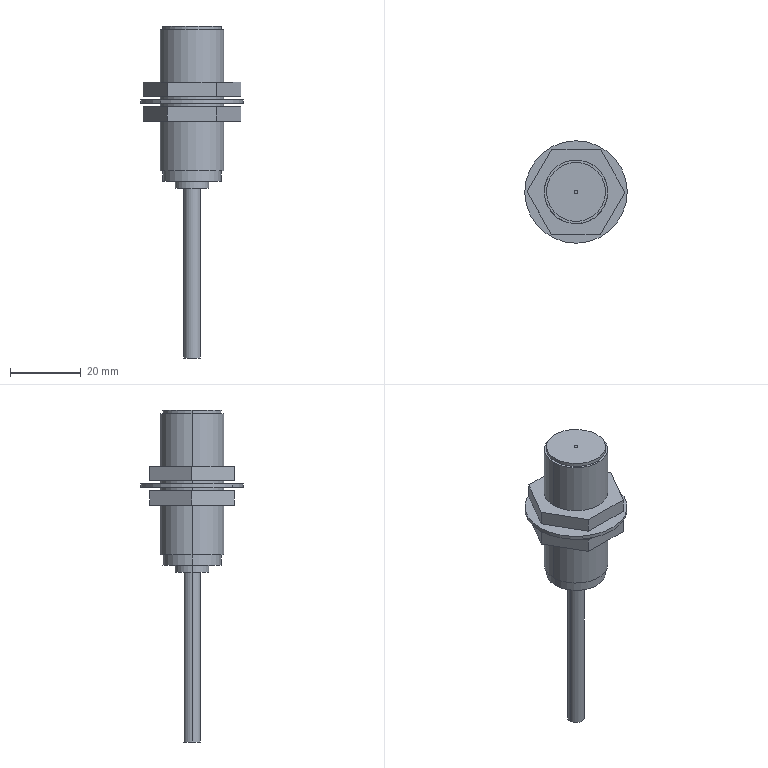Part | STEP file | gx-118m | 4 solids | 60 faces | box 29 x 29 x 94 mm | volume 14418 mm3 | cylinder 30 | plane 30 | commonest cylinder face diameters 1 x12 18 x8 4.8 x2 9.5 x2 16.6 x2 16.7 x2